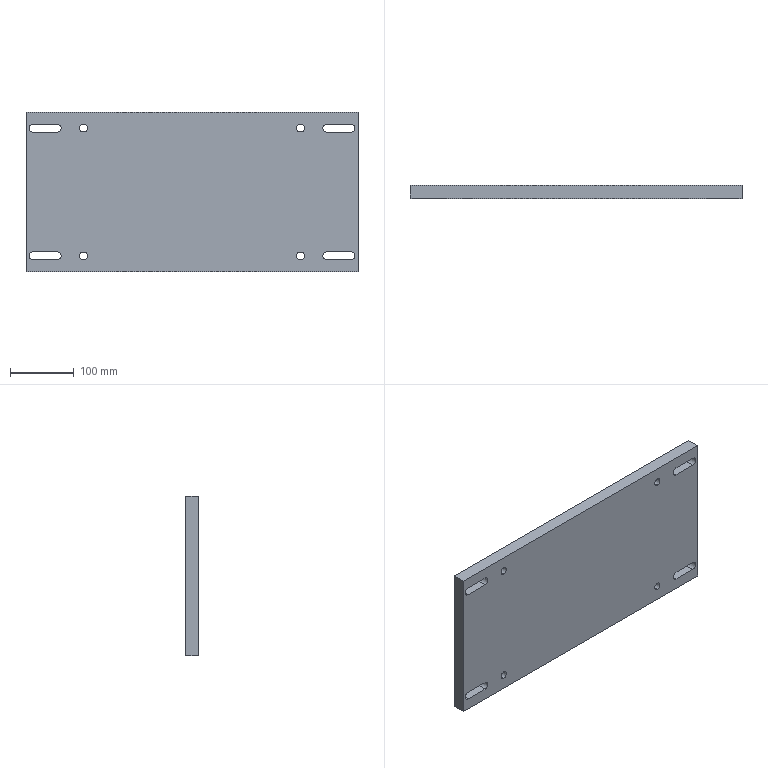Part | STEP file | Motor mounting plate | 1 solid | 30 faces | box 520 x 20 x 250 mm | volume 2541854 mm3 | cylinder 16 | plane 14 | commonest cylinder face diameters 12 x8 13 x8